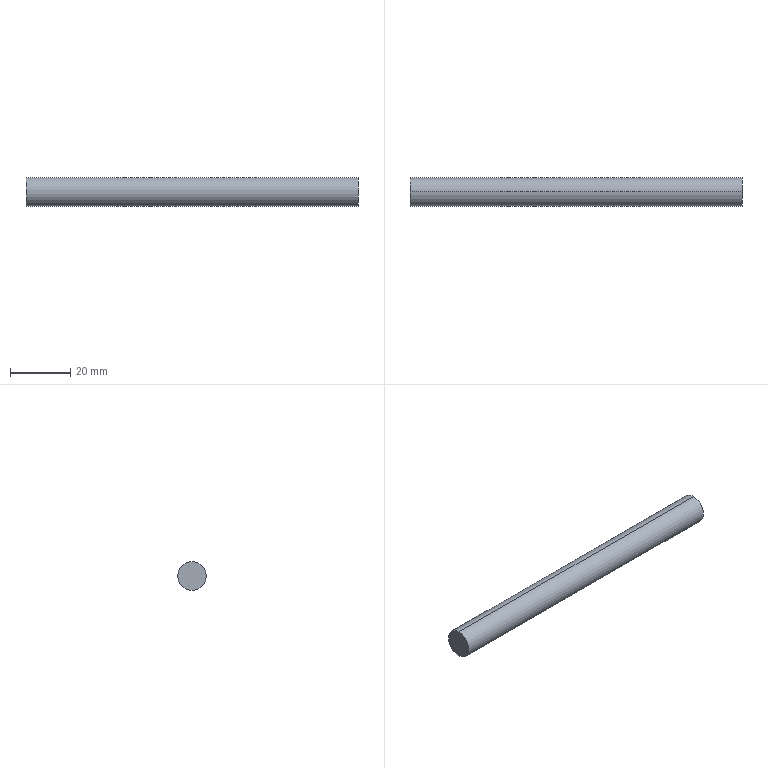Part | STEP file | 4-20.sldasm-Part-104 | 1 solid | 4 faces | box 110 x 9.525 x 9.525 mm | volume 7838 mm3 | cylinder 2 | plane 2 | commonest cylinder face diameters 9.525 x2
STEP:
#1=CARTESIAN_POINT('',(128.125,47.,20.762));
#2=VERTEX_POINT('',#1);
#3=CARTESIAN_POINT('',(128.125,47.,11.238));
#4=VERTEX_POINT('',#3);
#5=CARTESIAN_POINT('',(128.125,47.,16.));
#6=DIRECTION('',(-1.,0.,0.));
#7=DIRECTION('',(0.,0.,-1.));
#8=AXIS2_PLACEMENT_3D('',#5,#6,#7);
#9=CIRCLE('',#8,4.762);
#10=EDGE_CURVE('',#2,#4,#9,.T.);
#11=ORIENTED_EDGE('',*,*,#10,.F.);
#12=CARTESIAN_POINT('',(238.125,47.,20.762));
#13=VERTEX_POINT('',#12);
#14=CARTESIAN_POINT('',(-431.8,47.,20.762));
#15=DIRECTION('',(1.,0.,0.));
#16=VECTOR('',#15,1000.);
#17=LINE('',#14,#16);
#18=EDGE_CURVE('',#2,#13,#17,.T.);
#19=ORIENTED_EDGE('',*,*,#18,.T.);
#20=CARTESIAN_POINT('',(238.125,47.,11.238));
#21=VERTEX_POINT('',#20);
#22=CARTESIAN_POINT('',(238.125,47.,16.));
#23=DIRECTION('',(1.,0.,0.));
#24=DIRECTION('',(0.,0.,1.));
#25=AXIS2_PLACEMENT_3D('',#22,#23,#24);
#26=CIRCLE('',#25,4.762);
#27=EDGE_CURVE('',#21,#13,#26,.T.);
#28=ORIENTED_EDGE('',*,*,#27,.F.);
#29=CARTESIAN_POINT('',(-431.8,47.,11.238));
#30=DIRECTION('',(1.,0.,0.));
#31=VECTOR('',#30,1000.);
#32=LINE('',#29,#31);
#33=EDGE_CURVE('',#4,#21,#32,.T.);
#34=ORIENTED_EDGE('',*,*,#33,.F.);
#35=EDGE_LOOP('',(#11,#19,#28,#34));
#36=FACE_OUTER_BOUND('',#35,.T.);
#37=CARTESIAN_POINT('',(-431.8,47.,16.));
#38=DIRECTION('',(1.,0.,0.));
#39=DIRECTION('',(0.,0.,-1.));
#40=AXIS2_PLACEMENT_3D('',#37,#38,#39);
#41=CYLINDRICAL_SURFACE('',#40,4.762);
#42=ADVANCED_FACE('',(#36),#41,.T.);
#43=ORIENTED_EDGE('',*,*,#27,.T.);
#44=CARTESIAN_POINT('',(238.125,47.,16.));
#45=DIRECTION('',(1.,0.,0.));
#46=DIRECTION('',(0.,0.,1.));
#47=AXIS2_PLACEMENT_3D('',#44,#45,#46);
#48=CIRCLE('',#47,4.762);
#49=EDGE_CURVE('',#13,#21,#48,.T.);
#50=ORIENTED_EDGE('',*,*,#49,.T.);
#51=EDGE_LOOP('',(#43,#50));
#52=FACE_OUTER_BOUND('',#51,.T.);
#53=CARTESIAN_POINT('',(238.125,-340.,62.));
#54=DIRECTION('',(-1.,0.,0.));
#55=DIRECTION('',(0.,0.,1.));
#56=AXIS2_PLACEMENT_3D('',#53,#54,#55);
#57=PLANE('',#56);
#58=ADVANCED_FACE('',(#52),#57,.F.);
#59=ORIENTED_EDGE('',*,*,#18,.F.);
#60=CARTESIAN_POINT('',(128.125,47.,16.));
#61=DIRECTION('',(-1.,0.,0.));
#62=DIRECTION('',(0.,0.,-1.));
#63=AXIS2_PLACEMENT_3D('',#60,#61,#62);
#64=CIRCLE('',#63,4.762);
#65=EDGE_CURVE('',#4,#2,#64,.T.);
#66=ORIENTED_EDGE('',*,*,#65,.F.);
#67=ORIENTED_EDGE('',*,*,#33,.T.);
#68=ORIENTED_EDGE('',*,*,#49,.F.);
#69=EDGE_LOOP('',(#59,#66,#67,#68));
#70=FACE_OUTER_BOUND('',#69,.T.);
#71=CARTESIAN_POINT('',(-431.8,47.,16.));
#72=DIRECTION('',(1.,0.,0.));
#73=DIRECTION('',(0.,0.,-1.));
#74=AXIS2_PLACEMENT_3D('',#71,#72,#73);
#75=CYLINDRICAL_SURFACE('',#74,4.762);
#76=ADVANCED_FACE('',(#70),#75,.T.);
#77=ORIENTED_EDGE('',*,*,#65,.T.);
#78=ORIENTED_EDGE('',*,*,#10,.T.);
#79=EDGE_LOOP('',(#77,#78));
#80=FACE_OUTER_BOUND('',#79,.T.);
#81=CARTESIAN_POINT('',(128.125,491.8,16.));
#82=DIRECTION('',(1.,0.,0.));
#83=DIRECTION('',(0.,0.,-1.));
#84=AXIS2_PLACEMENT_3D('',#81,#82,#83);
#85=PLANE('',#84);
#86=ADVANCED_FACE('',(#80),#85,.F.);
#87=CLOSED_SHELL('',(#42,#58,#76,#86));
#88=MANIFOLD_SOLID_BREP('',#87);
#89=CARTESIAN_POINT('',(0.,0.,0.));
#90=DIRECTION('',(0.,0.,1.));
#91=DIRECTION('',(1.,0.,0.));
#92=AXIS2_PLACEMENT_3D('',#89,#90,#91);
#93=(LENGTH_UNIT()NAMED_UNIT(*)SI_UNIT(.MILLI.,.METRE.));
#94=UNCERTAINTY_MEASURE_WITH_UNIT(LENGTH_MEASURE(0.00001),#93,'','');
#95=(NAMED_UNIT(*)PLANE_ANGLE_UNIT()SI_UNIT($,.RADIAN.));
#96=(NAMED_UNIT(*)SI_UNIT($,.STERADIAN.)SOLID_ANGLE_UNIT());
#97=(GEOMETRIC_REPRESENTATION_CONTEXT(3)GLOBAL_UNCERTAINTY_ASSIGNED_CONTEXT((#94))GLOBAL_UNIT_ASSIGNED_CONTEXT((#93,#95,#96))REPRESENTATION_CONTEXT('',''));
#98=ADVANCED_BREP_SHAPE_REPRESENTATION('',(#88,#92),#97);